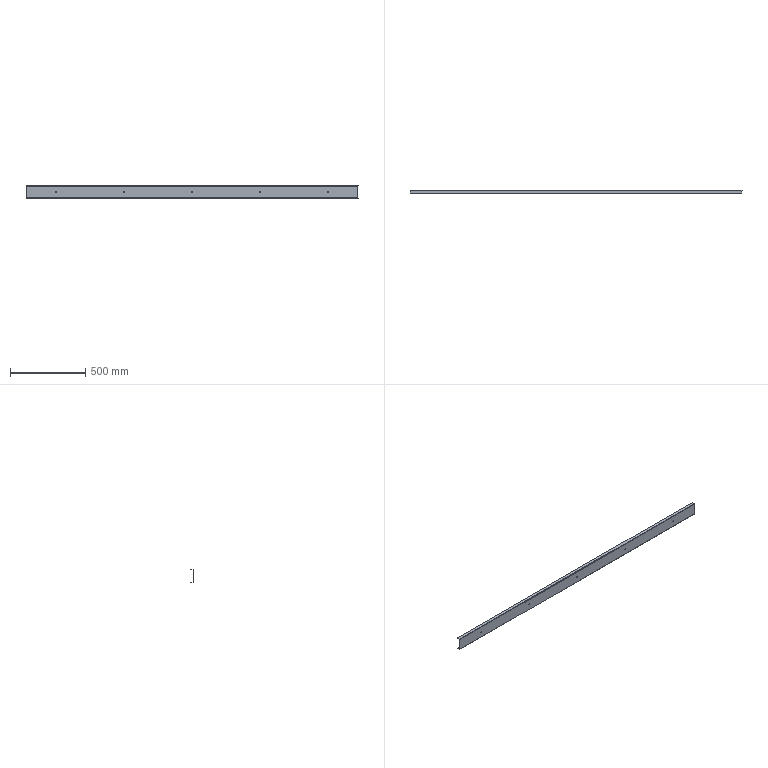Part | SolidWorks | features EdgeFlange 1, FlatPattern 1, HoleWzd 1, SMBaseFlange 1, SheetMetal 1 | 1 solid | 32 faces | box 2200 x 22 x 84 mm | volume 538758 mm3 | plane 18 | cylinder 14 | commonest cylinder face diameters 6 x10 1.473 x2 5.473 x2
STEP:
#1=CARTESIAN_POINT('',(900.,-2.,-3.));
#2=VERTEX_POINT('',#1);
#3=CARTESIAN_POINT('',(900.,-2.,3.));
#4=VERTEX_POINT('',#3);
#5=CARTESIAN_POINT('',(900.,-2.,0.));
#6=DIRECTION('',(0.,1.,0.));
#7=DIRECTION('',(0.,0.,1.));
#8=AXIS2_PLACEMENT_3D('',#5,#6,#7);
#9=CIRCLE('',#8,3.);
#10=EDGE_CURVE('',#2,#4,#9,.T.);
#11=ORIENTED_EDGE('',*,*,#10,.F.);
#12=CARTESIAN_POINT('',(900.,0.,-3.));
#13=VERTEX_POINT('',#12);
#14=CARTESIAN_POINT('',(900.,0.,-3.));
#15=DIRECTION('',(0.,1.,0.));
#16=VECTOR('',#15,1000.);
#17=LINE('',#14,#16);
#18=EDGE_CURVE('',#2,#13,#17,.T.);
#19=ORIENTED_EDGE('',*,*,#18,.T.);
#20=CARTESIAN_POINT('',(900.,0.,3.));
#21=VERTEX_POINT('',#20);
#22=CARTESIAN_POINT('',(900.,0.,0.));
#23=DIRECTION('',(0.,1.,0.));
#24=DIRECTION('',(0.,0.,1.));
#25=AXIS2_PLACEMENT_3D('',#22,#23,#24);
#26=CIRCLE('',#25,3.);
#27=EDGE_CURVE('',#13,#21,#26,.T.);
#28=ORIENTED_EDGE('',*,*,#27,.T.);
#29=CARTESIAN_POINT('',(900.,0.,3.));
#30=DIRECTION('',(0.,1.,0.));
#31=VECTOR('',#30,1000.);
#32=LINE('',#29,#31);
#33=EDGE_CURVE('',#4,#21,#32,.T.);
#34=ORIENTED_EDGE('',*,*,#33,.F.);
#35=EDGE_LOOP('',(#11,#19,#28,#34));
#36=FACE_OUTER_BOUND('',#35,.T.);
#37=CARTESIAN_POINT('',(900.,0.,0.));
#38=DIRECTION('',(0.,1.,0.));
#39=DIRECTION('',(0.,0.,1.));
#40=AXIS2_PLACEMENT_3D('',#37,#38,#39);
#41=CYLINDRICAL_SURFACE('',#40,3.);
#42=ADVANCED_FACE('',(#36),#41,.F.);
#43=CARTESIAN_POINT('',(450.,-2.,-3.));
#44=VERTEX_POINT('',#43);
#45=CARTESIAN_POINT('',(450.,-2.,3.));
#46=VERTEX_POINT('',#45);
#47=CARTESIAN_POINT('',(450.,-2.,0.));
#48=DIRECTION('',(0.,1.,0.));
#49=DIRECTION('',(0.,0.,1.));
#50=AXIS2_PLACEMENT_3D('',#47,#48,#49);
#51=CIRCLE('',#50,3.);
#52=EDGE_CURVE('',#44,#46,#51,.T.);
#53=ORIENTED_EDGE('',*,*,#52,.F.);
#54=CARTESIAN_POINT('',(450.,0.,-3.));
#55=VERTEX_POINT('',#54);
#56=CARTESIAN_POINT('',(450.,0.,-3.));
#57=DIRECTION('',(0.,1.,0.));
#58=VECTOR('',#57,1000.);
#59=LINE('',#56,#58);
#60=EDGE_CURVE('',#44,#55,#59,.T.);
#61=ORIENTED_EDGE('',*,*,#60,.T.);
#62=CARTESIAN_POINT('',(450.,0.,3.));
#63=VERTEX_POINT('',#62);
#64=CARTESIAN_POINT('',(450.,0.,0.));
#65=DIRECTION('',(0.,1.,0.));
#66=DIRECTION('',(0.,0.,1.));
#67=AXIS2_PLACEMENT_3D('',#64,#65,#66);
#68=CIRCLE('',#67,3.);
#69=EDGE_CURVE('',#55,#63,#68,.T.);
#70=ORIENTED_EDGE('',*,*,#69,.T.);
#71=CARTESIAN_POINT('',(450.,0.,3.));
#72=DIRECTION('',(0.,1.,0.));
#73=VECTOR('',#72,1000.);
#74=LINE('',#71,#73);
#75=EDGE_CURVE('',#46,#63,#74,.T.);
#76=ORIENTED_EDGE('',*,*,#75,.F.);
#77=EDGE_LOOP('',(#53,#61,#70,#76));
#78=FACE_OUTER_BOUND('',#77,.T.);
#79=CARTESIAN_POINT('',(450.,0.,0.));
#80=DIRECTION('',(0.,1.,0.));
#81=DIRECTION('',(0.,0.,1.));
#82=AXIS2_PLACEMENT_3D('',#79,#80,#81);
#83=CYLINDRICAL_SURFACE('',#82,3.);
#84=ADVANCED_FACE('',(#78),#83,.F.);
#85=CARTESIAN_POINT('',(0.,-2.,-3.));
#86=VERTEX_POINT('',#85);
#87=CARTESIAN_POINT('',(0.,-2.,3.));
#88=VERTEX_POINT('',#87);
#89=CARTESIAN_POINT('',(0.,-2.,0.));
#90=DIRECTION('',(0.,1.,0.));
#91=DIRECTION('',(0.,0.,1.));
#92=AXIS2_PLACEMENT_3D('',#89,#90,#91);
#93=CIRCLE('',#92,3.);
#94=EDGE_CURVE('',#86,#88,#93,.T.);
#95=ORIENTED_EDGE('',*,*,#94,.F.);
#96=CARTESIAN_POINT('',(0.,0.,-3.));
#97=VERTEX_POINT('',#96);
#98=CARTESIAN_POINT('',(0.,0.,-3.));
#99=DIRECTION('',(0.,1.,0.));
#100=VECTOR('',#99,1000.);
#101=LINE('',#98,#100);
#102=EDGE_CURVE('',#86,#97,#101,.T.);
#103=ORIENTED_EDGE('',*,*,#102,.T.);
#104=CARTESIAN_POINT('',(0.,0.,3.));
#105=VERTEX_POINT('',#104);
#106=CARTESIAN_POINT('',(0.,0.,0.));
#107=DIRECTION('',(0.,1.,0.));
#108=DIRECTION('',(0.,0.,1.));
#109=AXIS2_PLACEMENT_3D('',#106,#107,#108);
#110=CIRCLE('',#109,3.);
#111=EDGE_CURVE('',#97,#105,#110,.T.);
#112=ORIENTED_EDGE('',*,*,#111,.T.);
#113=CARTESIAN_POINT('',(0.,0.,3.));
#114=DIRECTION('',(0.,1.,0.));
#115=VECTOR('',#114,1000.);
#116=LINE('',#113,#115);
#117=EDGE_CURVE('',#88,#105,#116,.T.);
#118=ORIENTED_EDGE('',*,*,#117,.F.);
#119=EDGE_LOOP('',(#95,#103,#112,#118));
#120=FACE_OUTER_BOUND('',#119,.T.);
#121=CARTESIAN_POINT('',(0.,0.,0.));
#122=DIRECTION('',(0.,1.,0.));
#123=DIRECTION('',(0.,0.,1.));
#124=AXIS2_PLACEMENT_3D('',#121,#122,#123);
#125=CYLINDRICAL_SURFACE('',#124,3.);
#126=ADVANCED_FACE('',(#120),#125,.F.);
#127=CARTESIAN_POINT('',(-450.,-2.,-3.));
#128=VERTEX_POINT('',#127);
#129=CARTESIAN_POINT('',(-450.,-2.,3.));
#130=VERTEX_POINT('',#129);
#131=CARTESIAN_POINT('',(-450.,-2.,0.));
#132=DIRECTION('',(0.,1.,0.));
#133=DIRECTION('',(0.,0.,1.));
#134=AXIS2_PLACEMENT_3D('',#131,#132,#133);
#135=CIRCLE('',#134,3.);
#136=EDGE_CURVE('',#128,#130,#135,.T.);
#137=ORIENTED_EDGE('',*,*,#136,.F.);
#138=CARTESIAN_POINT('',(-450.,0.,-3.));
#139=VERTEX_POINT('',#138);
#140=CARTESIAN_POINT('',(-450.,0.,-3.));
#141=DIRECTION('',(0.,1.,0.));
#142=VECTOR('',#141,1000.);
#143=LINE('',#140,#142);
#144=EDGE_CURVE('',#128,#139,#143,.T.);
#145=ORIENTED_EDGE('',*,*,#144,.T.);
#146=CARTESIAN_POINT('',(-450.,0.,3.));
#147=VERTEX_POINT('',#146);
#148=CARTESIAN_POINT('',(-450.,0.,0.));
#149=DIRECTION('',(0.,1.,0.));
#150=DIRECTION('',(0.,0.,1.));
#151=AXIS2_PLACEMENT_3D('',#148,#149,#150);
#152=CIRCLE('',#151,3.);
#153=EDGE_CURVE('',#139,#147,#152,.T.);
#154=ORIENTED_EDGE('',*,*,#153,.T.);
#155=CARTESIAN_POINT('',(-450.,0.,3.));
#156=DIRECTION('',(0.,1.,0.));
#157=VECTOR('',#156,1000.);
#158=LINE('',#155,#157);
#159=EDGE_CURVE('',#130,#147,#158,.T.);
#160=ORIENTED_EDGE('',*,*,#159,.F.);
#161=EDGE_LOOP('',(#137,#145,#154,#160));
#162=FACE_OUTER_BOUND('',#161,.T.);
#163=CARTESIAN_POINT('',(-450.,0.,0.));
#164=DIRECTION('',(0.,1.,0.));
#165=DIRECTION('',(0.,0.,1.));
#166=AXIS2_PLACEMENT_3D('',#163,#164,#165);
#167=CYLINDRICAL_SURFACE('',#166,3.);
#168=ADVANCED_FACE('',(#162),#167,.F.);
#169=CARTESIAN_POINT('',(-900.,-2.,-3.));
#170=VERTEX_POINT('',#169);
#171=CARTESIAN_POINT('',(-900.,-2.,3.));
#172=VERTEX_POINT('',#171);
#173=CARTESIAN_POINT('',(-900.,-2.,0.));
#174=DIRECTION('',(0.,1.,0.));
#175=DIRECTION('',(0.,0.,1.));
#176=AXIS2_PLACEMENT_3D('',#173,#174,#175);
#177=CIRCLE('',#176,3.);
#178=EDGE_CURVE('',#170,#172,#177,.T.);
#179=ORIENTED_EDGE('',*,*,#178,.F.);
#180=CARTESIAN_POINT('',(-900.,0.,-3.));
#181=VERTEX_POINT('',#180);
#182=CARTESIAN_POINT('',(-900.,0.,-3.));
#183=DIRECTION('',(0.,1.,0.));
#184=VECTOR('',#183,1000.);
#185=LINE('',#182,#184);
#186=EDGE_CURVE('',#170,#181,#185,.T.);
#187=ORIENTED_EDGE('',*,*,#186,.T.);
#188=CARTESIAN_POINT('',(-900.,0.,3.));
#189=VERTEX_POINT('',#188);
#190=CARTESIAN_POINT('',(-900.,0.,0.));
#191=DIRECTION('',(0.,1.,0.));
#192=DIRECTION('',(0.,0.,1.));
#193=AXIS2_PLACEMENT_3D('',#190,#191,#192);
#194=CIRCLE('',#193,3.);
#195=EDGE_CURVE('',#181,#189,#194,.T.);
#196=ORIENTED_EDGE('',*,*,#195,.T.);
#197=CARTESIAN_POINT('',(-900.,0.,3.));
#198=DIRECTION('',(0.,1.,0.));
#199=VECTOR('',#198,1000.);
#200=LINE('',#197,#199);
#201=EDGE_CURVE('',#172,#189,#200,.T.);
#202=ORIENTED_EDGE('',*,*,#201,.F.);
#203=EDGE_LOOP('',(#179,#187,#196,#202));
#204=FACE_OUTER_BOUND('',#203,.T.);
#205=CARTESIAN_POINT('',(-900.,0.,0.));
#206=DIRECTION('',(0.,1.,0.));
#207=DIRECTION('',(0.,0.,1.));
#208=AXIS2_PLACEMENT_3D('',#205,#206,#207);
#209=CYLINDRICAL_SURFACE('',#208,3.);
#210=ADVANCED_FACE('',(#204),#209,.F.);
#211=CARTESIAN_POINT('',(900.,-2.,0.));
#212=DIRECTION('',(0.,1.,0.));
#213=DIRECTION('',(0.,0.,1.));
#214=AXIS2_PLACEMENT_3D('',#211,#212,#213);
#215=CIRCLE('',#214,3.);
#216=EDGE_CURVE('',#4,#2,#215,.T.);
#217=ORIENTED_EDGE('',*,*,#216,.T.);
#218=ORIENTED_EDGE('',*,*,#10,.T.);
#219=EDGE_LOOP('',(#217,#218));
#220=FACE_BOUND('',#219,.T.);
#221=CARTESIAN_POINT('',(450.,-2.,0.));
#222=DIRECTION('',(0.,1.,0.));
#223=DIRECTION('',(0.,0.,1.));
#224=AXIS2_PLACEMENT_3D('',#221,#222,#223);
#225=CIRCLE('',#224,3.);
#226=EDGE_CURVE('',#46,#44,#225,.T.);
#227=ORIENTED_EDGE('',*,*,#226,.T.);
#228=ORIENTED_EDGE('',*,*,#52,.T.);
#229=EDGE_LOOP('',(#227,#228));
#230=FACE_BOUND('',#229,.T.);
#231=CARTESIAN_POINT('',(0.,-2.,0.));
#232=DIRECTION('',(0.,1.,0.));
#233=DIRECTION('',(0.,0.,1.));
#234=AXIS2_PLACEMENT_3D('',#231,#232,#233);
#235=CIRCLE('',#234,3.);
#236=EDGE_CURVE('',#88,#86,#235,.T.);
#237=ORIENTED_EDGE('',*,*,#236,.T.);
#238=ORIENTED_EDGE('',*,*,#94,.T.);
#239=EDGE_LOOP('',(#237,#238));
#240=FACE_BOUND('',#239,.T.);
#241=CARTESIAN_POINT('',(-450.,-2.,0.));
#242=DIRECTION('',(0.,1.,0.));
#243=DIRECTION('',(0.,0.,1.));
#244=AXIS2_PLACEMENT_3D('',#241,#242,#243);
#245=CIRCLE('',#244,3.);
#246=EDGE_CURVE('',#130,#128,#245,.T.);
#247=ORIENTED_EDGE('',*,*,#246,.T.);
#248=ORIENTED_EDGE('',*,*,#136,.T.);
#249=EDGE_LOOP('',(#247,#248));
#250=FACE_BOUND('',#249,.T.);
#251=CARTESIAN_POINT('',(-900.,-2.,0.));
#252=DIRECTION('',(0.,1.,0.));
#253=DIRECTION('',(0.,0.,1.));
#254=AXIS2_PLACEMENT_3D('',#251,#252,#253);
#255=CIRCLE('',#254,3.);
#256=EDGE_CURVE('',#172,#170,#255,.T.);
#257=ORIENTED_EDGE('',*,*,#256,.T.);
#258=ORIENTED_EDGE('',*,*,#178,.T.);
#259=EDGE_LOOP('',(#257,#258));
#260=FACE_BOUND('',#259,.T.);
#261=CARTESIAN_POINT('',(-1100.,-2.,-39.263));
#262=VERTEX_POINT('',#261);
#263=CARTESIAN_POINT('',(1100.,-2.,-39.263));
#264=VERTEX_POINT('',#263);
#265=CARTESIAN_POINT('',(-1100.,-2.,-39.263));
#266=DIRECTION('',(1.,0.,0.));
#267=VECTOR('',#266,1000.);
#268=LINE('',#265,#267);
#269=EDGE_CURVE('',#262,#264,#268,.T.);
#270=ORIENTED_EDGE('',*,*,#269,.T.);
#271=CARTESIAN_POINT('',(1100.,-2.,39.263));
#272=VERTEX_POINT('',#271);
#273=CARTESIAN_POINT('',(1100.,-2.,-42.));
#274=DIRECTION('',(0.,0.,-1.));
#275=VECTOR('',#274,1000.);
#276=LINE('',#273,#275);
#277=EDGE_CURVE('',#272,#264,#276,.T.);
#278=ORIENTED_EDGE('',*,*,#277,.F.);
#279=CARTESIAN_POINT('',(-1100.,-2.,39.263));
#280=VERTEX_POINT('',#279);
#281=CARTESIAN_POINT('',(1100.,-2.,39.263));
#282=DIRECTION('',(-1.,0.,0.));
#283=VECTOR('',#282,1000.);
#284=LINE('',#281,#283);
#285=EDGE_CURVE('',#272,#280,#284,.T.);
#286=ORIENTED_EDGE('',*,*,#285,.T.);
#287=CARTESIAN_POINT('',(-1100.,-2.,-42.));
#288=DIRECTION('',(0.,0.,1.));
#289=VECTOR('',#288,1000.);
#290=LINE('',#287,#289);
#291=EDGE_CURVE('',#262,#280,#290,.T.);
#292=ORIENTED_EDGE('',*,*,#291,.F.);
#293=EDGE_LOOP('',(#270,#278,#286,#292));
#294=FACE_OUTER_BOUND('',#293,.T.);
#295=CARTESIAN_POINT('',(0.,-2.,0.));
#296=DIRECTION('',(0.,1.,0.));
#297=DIRECTION('',(0.,0.,1.));
#298=AXIS2_PLACEMENT_3D('',#295,#296,#297);
#299=PLANE('',#298);
#300=ADVANCED_FACE('',(#220,#230,#240,#250,#260,#294),#299,.F.);
#301=CARTESIAN_POINT('',(900.,0.,0.));
#302=DIRECTION('',(0.,1.,0.));
#303=DIRECTION('',(0.,0.,1.));
#304=AXIS2_PLACEMENT_3D('',#301,#302,#303);
#305=CIRCLE('',#304,3.);
#306=EDGE_CURVE('',#21,#13,#305,.T.);
#307=ORIENTED_EDGE('',*,*,#306,.F.);
#308=ORIENTED_EDGE('',*,*,#27,.F.);
#309=EDGE_LOOP('',(#307,#308));
#310=FACE_BOUND('',#309,.T.);
#311=CARTESIAN_POINT('',(450.,0.,0.));
#312=DIRECTION('',(0.,1.,0.));
#313=DIRECTION('',(0.,0.,1.));
#314=AXIS2_PLACEMENT_3D('',#311,#312,#313);
#315=CIRCLE('',#314,3.);
#316=EDGE_CURVE('',#63,#55,#315,.T.);
#317=ORIENTED_EDGE('',*,*,#316,.F.);
#318=ORIENTED_EDGE('',*,*,#69,.F.);
#319=EDGE_LOOP('',(#317,#318));
#320=FACE_BOUND('',#319,.T.);
#321=CARTESIAN_POINT('',(0.,0.,0.));
#322=DIRECTION('',(0.,1.,0.));
#323=DIRECTION('',(0.,0.,1.));
#324=AXIS2_PLACEMENT_3D('',#321,#322,#323);
#325=CIRCLE('',#324,3.);
#326=EDGE_CURVE('',#105,#97,#325,.T.);
#327=ORIENTED_EDGE('',*,*,#326,.F.);
#328=ORIENTED_EDGE('',*,*,#111,.F.);
#329=EDGE_LOOP('',(#327,#328));
#330=FACE_BOUND('',#329,.T.);
#331=CARTESIAN_POINT('',(-450.,0.,0.));
#332=DIRECTION('',(0.,1.,0.));
#333=DIRECTION('',(0.,0.,1.));
#334=AXIS2_PLACEMENT_3D('',#331,#332,#333);
#335=CIRCLE('',#334,3.);
#336=EDGE_CURVE('',#147,#139,#335,.T.);
#337=ORIENTED_EDGE('',*,*,#336,.F.);
#338=ORIENTED_EDGE('',*,*,#153,.F.);
#339=EDGE_LOOP('',(#337,#338));
#340=FACE_BOUND('',#339,.T.);
#341=CARTESIAN_POINT('',(-900.,0.,0.));
#342=DIRECTION('',(0.,1.,0.));
#343=DIRECTION('',(0.,0.,1.));
#344=AXIS2_PLACEMENT_3D('',#341,#342,#343);
#345=CIRCLE('',#344,3.);
#346=EDGE_CURVE('',#189,#181,#345,.T.);
#347=ORIENTED_EDGE('',*,*,#346,.F.);
#348=ORIENTED_EDGE('',*,*,#195,.F.);
#349=EDGE_LOOP('',(#347,#348));
#350=FACE_BOUND('',#349,.T.);
#351=CARTESIAN_POINT('',(1100.,0.,39.263));
#352=VERTEX_POINT('',#351);
#353=CARTESIAN_POINT('',(1100.,0.,-39.263));
#354=VERTEX_POINT('',#353);
#355=CARTESIAN_POINT('',(1100.,0.,-42.));
#356=DIRECTION('',(0.,0.,-1.));
#357=VECTOR('',#356,1000.);
#358=LINE('',#355,#357);
#359=EDGE_CURVE('',#352,#354,#358,.T.);
#360=ORIENTED_EDGE('',*,*,#359,.T.);
#361=CARTESIAN_POINT('',(-1100.,0.,-39.263));
#362=VERTEX_POINT('',#361);
#363=CARTESIAN_POINT('',(-1100.,0.,-39.263));
#364=DIRECTION('',(1.,0.,0.));
#365=VECTOR('',#364,1000.);
#366=LINE('',#363,#365);
#367=EDGE_CURVE('',#362,#354,#366,.T.);
#368=ORIENTED_EDGE('',*,*,#367,.F.);
#369=CARTESIAN_POINT('',(-1100.,0.,39.263));
#370=VERTEX_POINT('',#369);
#371=CARTESIAN_POINT('',(-1100.,0.,-42.));
#372=DIRECTION('',(0.,0.,1.));
#373=VECTOR('',#372,1000.);
#374=LINE('',#371,#373);
#375=EDGE_CURVE('',#362,#370,#374,.T.);
#376=ORIENTED_EDGE('',*,*,#375,.T.);
#377=CARTESIAN_POINT('',(1100.,0.,39.263));
#378=DIRECTION('',(-1.,0.,0.));
#379=VECTOR('',#378,1000.);
#380=LINE('',#377,#379);
#381=EDGE_CURVE('',#352,#370,#380,.T.);
#382=ORIENTED_EDGE('',*,*,#381,.F.);
#383=EDGE_LOOP('',(#360,#368,#376,#382));
#384=FACE_OUTER_BOUND('',#383,.T.);
#385=CARTESIAN_POINT('',(0.,0.,0.));
#386=DIRECTION('',(0.,1.,0.));
#387=DIRECTION('',(0.,0.,1.));
#388=AXIS2_PLACEMENT_3D('',#385,#386,#387);
#389=PLANE('',#388);
#390=ADVANCED_FACE('',(#310,#320,#330,#340,#350,#384),#389,.T.);
#391=ORIENTED_EDGE('',*,*,#375,.F.);
#392=CARTESIAN_POINT('',(-1100.,0.,-39.263));
#393=DIRECTION('',(0.,-1.,0.));
#394=VECTOR('',#393,1000.);
#395=LINE('',#392,#394);
#396=EDGE_CURVE('',#362,#262,#395,.T.);
#397=ORIENTED_EDGE('',*,*,#396,.T.);
#398=ORIENTED_EDGE('',*,*,#291,.T.);
#399=CARTESIAN_POINT('',(-1100.,0.,39.263));
#400=DIRECTION('',(0.,-1.,0.));
#401=VECTOR('',#400,1000.);
#402=LINE('',#399,#401);
#403=EDGE_CURVE('',#370,#280,#402,.T.);
#404=ORIENTED_EDGE('',*,*,#403,.F.);
#405=EDGE_LOOP('',(#391,#397,#398,#404));
#406=FACE_OUTER_BOUND('',#405,.T.);
#407=CARTESIAN_POINT('',(-1100.,-2.,-42.));
#408=DIRECTION('',(-1.,0.,0.));
#409=DIRECTION('',(0.,0.,1.));
#410=AXIS2_PLACEMENT_3D('',#407,#408,#409);
#411=PLANE('',#410);
#412=ADVANCED_FACE('',(#406),#411,.T.);
#413=CARTESIAN_POINT('',(1100.,0.,-39.263));
#414=DIRECTION('',(0.,-1.,0.));
#415=VECTOR('',#414,1000.);
#416=LINE('',#413,#415);
#417=EDGE_CURVE('',#354,#264,#416,.T.);
#418=ORIENTED_EDGE('',*,*,#417,.F.);
#419=ORIENTED_EDGE('',*,*,#359,.F.);
#420=CARTESIAN_POINT('',(1100.,0.,39.263));
#421=DIRECTION('',(0.,-1.,0.));
#422=VECTOR('',#421,1000.);
#423=LINE('',#420,#422);
#424=EDGE_CURVE('',#352,#272,#423,.T.);
#425=ORIENTED_EDGE('',*,*,#424,.T.);
#426=ORIENTED_EDGE('',*,*,#277,.T.);
#427=EDGE_LOOP('',(#418,#419,#425,#426));
#428=FACE_OUTER_BOUND('',#427,.T.);
#429=CARTESIAN_POINT('',(1100.,-2.,-42.));
#430=DIRECTION('',(1.,0.,0.));
#431=DIRECTION('',(0.,0.,-1.));
#432=AXIS2_PLACEMENT_3D('',#429,#430,#431);
#433=PLANE('',#432);
#434=ADVANCED_FACE('',(#428),#433,.T.);
#435=CARTESIAN_POINT('',(-1100.,0.7366,40.));
#436=VERTEX_POINT('',#435);
#437=CARTESIAN_POINT('',(-1100.,0.7366,42.));
#438=VERTEX_POINT('',#437);
#439=CARTESIAN_POINT('',(-1100.,0.7366,42.));
#440=DIRECTION('',(0.,0.,1.));
#441=VECTOR('',#440,1000.);
#442=LINE('',#439,#441);
#443=EDGE_CURVE('',#436,#438,#442,.T.);
#444=ORIENTED_EDGE('',*,*,#443,.F.);
#445=CARTESIAN_POINT('',(-1100.,0.7366,39.263));
#446=DIRECTION('',(-1.,0.,0.));
#447=DIRECTION('',(0.,0.,-1.));
#448=AXIS2_PLACEMENT_3D('',#445,#446,#447);
#449=CIRCLE('',#448,0.7366);
#450=EDGE_CURVE('',#370,#436,#449,.T.);
#451=ORIENTED_EDGE('',*,*,#450,.F.);
#452=ORIENTED_EDGE('',*,*,#403,.T.);
#453=CARTESIAN_POINT('',(-1100.,0.7366,39.263));
#454=DIRECTION('',(-1.,0.,0.));
#455=DIRECTION('',(0.,0.,-1.));
#456=AXIS2_PLACEMENT_3D('',#453,#454,#455);
#457=CIRCLE('',#456,2.737);
#458=EDGE_CURVE('',#280,#438,#457,.T.);
#459=ORIENTED_EDGE('',*,*,#458,.T.);
#460=EDGE_LOOP('',(#444,#451,#452,#459));
#461=FACE_OUTER_BOUND('',#460,.T.);
#462=CARTESIAN_POINT('',(-1100.,0.7366,39.263));
#463=DIRECTION('',(-1.,0.,0.));
#464=DIRECTION('',(0.,0.,1.));
#465=AXIS2_PLACEMENT_3D('',#462,#463,#464);
#466=PLANE('',#465);
#467=ADVANCED_FACE('',(#461),#466,.T.);
#468=CARTESIAN_POINT('',(1100.,0.7366,40.));
#469=VERTEX_POINT('',#468);
#470=CARTESIAN_POINT('',(1100.,0.7366,39.263));
#471=DIRECTION('',(1.,0.,0.));
#472=DIRECTION('',(0.,0.,-1.));
#473=AXIS2_PLACEMENT_3D('',#470,#471,#472);
#474=CIRCLE('',#473,0.7366);
#475=EDGE_CURVE('',#469,#352,#474,.T.);
#476=ORIENTED_EDGE('',*,*,#475,.F.);
#477=CARTESIAN_POINT('',(1100.,0.7366,42.));
#478=VERTEX_POINT('',#477);
#479=CARTESIAN_POINT('',(1100.,0.7366,40.));
#480=DIRECTION('',(0.,0.,1.));
#481=VECTOR('',#480,1000.);
#482=LINE('',#479,#481);
#483=EDGE_CURVE('',#469,#478,#482,.T.);
#484=ORIENTED_EDGE('',*,*,#483,.T.);
#485=CARTESIAN_POINT('',(1100.,0.7366,39.263));
#486=DIRECTION('',(1.,0.,0.));
#487=DIRECTION('',(0.,0.,-1.));
#488=AXIS2_PLACEMENT_3D('',#485,#486,#487);
#489=CIRCLE('',#488,2.737);
#490=EDGE_CURVE('',#478,#272,#489,.T.);
#491=ORIENTED_EDGE('',*,*,#490,.T.);
#492=ORIENTED_EDGE('',*,*,#424,.F.);
#493=EDGE_LOOP('',(#476,#484,#491,#492));
#494=FACE_OUTER_BOUND('',#493,.T.);
#495=CARTESIAN_POINT('',(1100.,0.7366,39.263));
#496=DIRECTION('',(-1.,0.,0.));
#497=DIRECTION('',(0.,0.,1.));
#498=AXIS2_PLACEMENT_3D('',#495,#496,#497);
#499=PLANE('',#498);
#500=ADVANCED_FACE('',(#494),#499,.F.);
#501=ORIENTED_EDGE('',*,*,#285,.F.);
#502=ORIENTED_EDGE('',*,*,#490,.F.);
#503=CARTESIAN_POINT('',(-1100.,0.7366,42.));
#504=DIRECTION('',(-1.,0.,0.));
#505=VECTOR('',#504,1000.);
#506=LINE('',#503,#505);
#507=EDGE_CURVE('',#478,#438,#506,.T.);
#508=ORIENTED_EDGE('',*,*,#507,.T.);
#509=ORIENTED_EDGE('',*,*,#458,.F.);
#510=EDGE_LOOP('',(#501,#502,#508,#509));
#511=FACE_OUTER_BOUND('',#510,.T.);
#512=CARTESIAN_POINT('',(1100.,0.7366,39.263));
#513=DIRECTION('',(1.,0.,0.));
#514=DIRECTION('',(0.,0.,1.));
#515=AXIS2_PLACEMENT_3D('',#512,#513,#514);
#516=CYLINDRICAL_SURFACE('',#515,2.737);
#517=ADVANCED_FACE('',(#511),#516,.T.);
#518=ORIENTED_EDGE('',*,*,#381,.T.);
#519=ORIENTED_EDGE('',*,*,#450,.T.);
#520=CARTESIAN_POINT('',(-1100.,0.7366,40.));
#521=DIRECTION('',(1.,0.,0.));
#522=VECTOR('',#521,1000.);
#523=LINE('',#520,#522);
#524=EDGE_CURVE('',#436,#469,#523,.T.);
#525=ORIENTED_EDGE('',*,*,#524,.T.);
#526=ORIENTED_EDGE('',*,*,#475,.T.);
#527=EDGE_LOOP('',(#518,#519,#525,#526));
#528=FACE_OUTER_BOUND('',#527,.T.);
#529=CARTESIAN_POINT('',(1100.,0.7366,39.263));
#530=DIRECTION('',(1.,0.,0.));
#531=DIRECTION('',(0.,0.,1.));
#532=AXIS2_PLACEMENT_3D('',#529,#530,#531);
#533=CYLINDRICAL_SURFACE('',#532,0.7366);
#534=ADVANCED_FACE('',(#528),#533,.F.);
#535=ORIENTED_EDGE('',*,*,#443,.T.);
#536=CARTESIAN_POINT('',(-1100.,20.,42.));
#537=VERTEX_POINT('',#536);
#538=CARTESIAN_POINT('',(-1100.,0.,42.));
#539=DIRECTION('',(0.,-1.,0.));
#540=VECTOR('',#539,1000.);
#541=LINE('',#538,#540);
#542=EDGE_CURVE('',#537,#438,#541,.T.);
#543=ORIENTED_EDGE('',*,*,#542,.F.);
#544=CARTESIAN_POINT('',(-1100.,20.,40.));
#545=VERTEX_POINT('',#544);
#546=CARTESIAN_POINT('',(-1100.,20.,42.));
#547=DIRECTION('',(0.,0.,-1.));
#548=VECTOR('',#547,1000.);
#549=LINE('',#546,#548);
#550=EDGE_CURVE('',#537,#545,#549,.T.);
#551=ORIENTED_EDGE('',*,*,#550,.T.);
#552=CARTESIAN_POINT('',(-1100.,0.,40.));
#553=DIRECTION('',(0.,-1.,0.));
#554=VECTOR('',#553,1000.);
#555=LINE('',#552,#554);
#556=EDGE_CURVE('',#545,#436,#555,.T.);
#557=ORIENTED_EDGE('',*,*,#556,.T.);
#558=EDGE_LOOP('',(#535,#543,#551,#557));
#559=FACE_OUTER_BOUND('',#558,.T.);
#560=CARTESIAN_POINT('',(-1100.,0.,42.));
#561=DIRECTION('',(1.,0.,0.));
#562=DIRECTION('',(0.,1.,0.));
#563=AXIS2_PLACEMENT_3D('',#560,#561,#562);
#564=PLANE('',#563);
#565=ADVANCED_FACE('',(#559),#564,.F.);
#566=ORIENTED_EDGE('',*,*,#483,.F.);
#567=CARTESIAN_POINT('',(1100.,20.,40.));
#568=VERTEX_POINT('',#567);
#569=CARTESIAN_POINT('',(1100.,20.,40.));
#570=DIRECTION('',(0.,1.,0.));
#571=VECTOR('',#570,1000.);
#572=LINE('',#569,#571);
#573=EDGE_CURVE('',#469,#568,#572,.T.);
#574=ORIENTED_EDGE('',*,*,#573,.T.);
#575=CARTESIAN_POINT('',(1100.,20.,42.));
#576=VERTEX_POINT('',#575);
#577=CARTESIAN_POINT('',(1100.,20.,42.));
#578=DIRECTION('',(0.,0.,-1.));
#579=VECTOR('',#578,1000.);
#580=LINE('',#577,#579);
#581=EDGE_CURVE('',#576,#568,#580,.T.);
#582=ORIENTED_EDGE('',*,*,#581,.F.);
#583=CARTESIAN_POINT('',(1100.,0.,42.));
#584=DIRECTION('',(0.,1.,0.));
#585=VECTOR('',#584,1000.);
#586=LINE('',#583,#585);
#587=EDGE_CURVE('',#478,#576,#586,.T.);
#588=ORIENTED_EDGE('',*,*,#587,.F.);
#589=EDGE_LOOP('',(#566,#574,#582,#588));
#590=FACE_OUTER_BOUND('',#589,.T.);
#591=CARTESIAN_POINT('',(1100.,20.,42.));
#592=DIRECTION('',(-1.,0.,0.));
#593=DIRECTION('',(0.,-1.,0.));
#594=AXIS2_PLACEMENT_3D('',#591,#592,#593);
#595=PLANE('',#594);
#596=ADVANCED_FACE('',(#590),#595,.F.);
#597=ORIENTED_EDGE('',*,*,#507,.F.);
#598=ORIENTED_EDGE('',*,*,#587,.T.);
#599=CARTESIAN_POINT('',(0.,20.,42.));
#600=DIRECTION('',(-1.,0.,0.));
#601=VECTOR('',#600,1000.);
#602=LINE('',#599,#601);
#603=EDGE_CURVE('',#576,#537,#602,.T.);
#604=ORIENTED_EDGE('',*,*,#603,.T.);
#605=ORIENTED_EDGE('',*,*,#542,.T.);
#606=EDGE_LOOP('',(#597,#598,#604,#605));
#607=FACE_OUTER_BOUND('',#606,.T.);
#608=CARTESIAN_POINT('',(0.,0.,42.));
#609=DIRECTION('',(0.,0.,-1.));
#610=DIRECTION('',(-1.,0.,0.));
#611=AXIS2_PLACEMENT_3D('',#608,#609,#610);
#612=PLANE('',#611);
#613=ADVANCED_FACE('',(#607),#612,.F.);
#614=ORIENTED_EDGE('',*,*,#573,.F.);
#615=ORIENTED_EDGE('',*,*,#524,.F.);
#616=ORIENTED_EDGE('',*,*,#556,.F.);
#617=CARTESIAN_POINT('',(-1100.,20.,40.));
#618=DIRECTION('',(-1.,0.,0.));
#619=VECTOR('',#618,1000.);
#620=LINE('',#617,#619);
#621=EDGE_CURVE('',#568,#545,#620,.T.);
#622=ORIENTED_EDGE('',*,*,#621,.F.);
#623=EDGE_LOOP('',(#614,#615,#616,#622));
#624=FACE_OUTER_BOUND('',#623,.T.);
#625=CARTESIAN_POINT('',(0.,0.,40.));
#626=DIRECTION('',(0.,0.,-1.));
#627=DIRECTION('',(-1.,0.,0.));
#628=AXIS2_PLACEMENT_3D('',#625,#626,#627);
#629=PLANE('',#628);
#630=ADVANCED_FACE('',(#624),#629,.T.);
#631=ORIENTED_EDGE('',*,*,#621,.T.);
#632=ORIENTED_EDGE('',*,*,#550,.F.);
#633=ORIENTED_EDGE('',*,*,#603,.F.);
#634=ORIENTED_EDGE('',*,*,#581,.T.);
#635=EDGE_LOOP('',(#631,#632,#633,#634));
#636=FACE_OUTER_BOUND('',#635,.T.);
#637=CARTESIAN_POINT('',(-1100.,20.,42.));
#638=DIRECTION('',(0.,-1.,0.));
#639=DIRECTION('',(0.,0.,-1.));
#640=AXIS2_PLACEMENT_3D('',#637,#638,#639);
#641=PLANE('',#640);
#642=ADVANCED_FACE('',(#636),#641,.F.);
#643=CARTESIAN_POINT('',(1100.,0.7366,-40.));
#644=VERTEX_POINT('',#643);
#645=CARTESIAN_POINT('',(1100.,0.7366,-42.));
#646=VERTEX_POINT('',#645);
#647=CARTESIAN_POINT('',(1100.,0.7366,-42.));
#648=DIRECTION('',(0.,0.,-1.));
#649=VECTOR('',#648,1000.);
#650=LINE('',#647,#649);
#651=EDGE_CURVE('',#644,#646,#650,.T.);
#652=ORIENTED_EDGE('',*,*,#651,.F.);
#653=CARTESIAN_POINT('',(1100.,0.7366,-39.263));
#654=DIRECTION('',(1.,0.,0.));
#655=DIRECTION('',(0.,-1.,0.));
#656=AXIS2_PLACEMENT_3D('',#653,#654,#655);
#657=CIRCLE('',#656,0.7366);
#658=EDGE_CURVE('',#354,#644,#657,.T.);
#659=ORIENTED_EDGE('',*,*,#658,.F.);
#660=ORIENTED_EDGE('',*,*,#417,.T.);
#661=CARTESIAN_POINT('',(1100.,0.7366,-39.263));
#662=DIRECTION('',(1.,0.,0.));
#663=DIRECTION('',(0.,-1.,0.));
#664=AXIS2_PLACEMENT_3D('',#661,#662,#663);
#665=CIRCLE('',#664,2.737);
#666=EDGE_CURVE('',#264,#646,#665,.T.);
#667=ORIENTED_EDGE('',*,*,#666,.T.);
#668=EDGE_LOOP('',(#652,#659,#660,#667));
#669=FACE_OUTER_BOUND('',#668,.T.);
#670=CARTESIAN_POINT('',(1100.,0.7366,-39.263));
#671=DIRECTION('',(1.,0.,0.));
#672=DIRECTION('',(0.,1.,0.));
#673=AXIS2_PLACEMENT_3D('',#670,#671,#672);
#674=PLANE('',#673);
#675=ADVANCED_FACE('',(#669),#674,.T.);
#676=CARTESIAN_POINT('',(-1100.,0.7366,-40.));
#677=VERTEX_POINT('',#676);
#678=CARTESIAN_POINT('',(-1100.,0.7366,-39.263));
#679=DIRECTION('',(-1.,0.,0.));
#680=DIRECTION('',(0.,-1.,0.));
#681=AXIS2_PLACEMENT_3D('',#678,#679,#680);
#682=CIRCLE('',#681,0.7366);
#683=EDGE_CURVE('',#677,#362,#682,.T.);
#684=ORIENTED_EDGE('',*,*,#683,.F.);
#685=CARTESIAN_POINT('',(-1100.,0.7366,-42.));
#686=VERTEX_POINT('',#685);
#687=CARTESIAN_POINT('',(-1100.,0.7366,-40.));
#688=DIRECTION('',(0.,0.,-1.));
#689=VECTOR('',#688,1000.);
#690=LINE('',#687,#689);
#691=EDGE_CURVE('',#677,#686,#690,.T.);
#692=ORIENTED_EDGE('',*,*,#691,.T.);
#693=CARTESIAN_POINT('',(-1100.,0.7366,-39.263));
#694=DIRECTION('',(-1.,0.,0.));
#695=DIRECTION('',(0.,-1.,0.));
#696=AXIS2_PLACEMENT_3D('',#693,#694,#695);
#697=CIRCLE('',#696,2.737);
#698=EDGE_CURVE('',#686,#262,#697,.T.);
#699=ORIENTED_EDGE('',*,*,#698,.T.);
#700=ORIENTED_EDGE('',*,*,#396,.F.);
#701=EDGE_LOOP('',(#684,#692,#699,#700));
#702=FACE_OUTER_BOUND('',#701,.T.);
#703=CARTESIAN_POINT('',(-1100.,0.7366,-39.263));
#704=DIRECTION('',(1.,0.,0.));
#705=DIRECTION('',(0.,1.,0.));
#706=AXIS2_PLACEMENT_3D('',#703,#704,#705);
#707=PLANE('',#706);
#708=ADVANCED_FACE('',(#702),#707,.F.);
#709=ORIENTED_EDGE('',*,*,#269,.F.);
#710=ORIENTED_EDGE('',*,*,#698,.F.);
#711=CARTESIAN_POINT('',(1100.,0.7366,-42.));
#712=DIRECTION('',(1.,0.,0.));
#713=VECTOR('',#712,1000.);
#714=LINE('',#711,#713);
#715=EDGE_CURVE('',#686,#646,#714,.T.);
#716=ORIENTED_EDGE('',*,*,#715,.T.);
#717=ORIENTED_EDGE('',*,*,#666,.F.);
#718=EDGE_LOOP('',(#709,#710,#716,#717));
#719=FACE_OUTER_BOUND('',#718,.T.);
#720=CARTESIAN_POINT('',(-1100.,0.7366,-39.263));
#721=DIRECTION('',(-1.,0.,0.));
#722=DIRECTION('',(0.,0.,-1.));
#723=AXIS2_PLACEMENT_3D('',#720,#721,#722);
#724=CYLINDRICAL_SURFACE('',#723,2.737);
#725=ADVANCED_FACE('',(#719),#724,.T.);
#726=ORIENTED_EDGE('',*,*,#367,.T.);
#727=ORIENTED_EDGE('',*,*,#658,.T.);
#728=CARTESIAN_POINT('',(1100.,0.7366,-40.));
#729=DIRECTION('',(-1.,0.,0.));
#730=VECTOR('',#729,1000.);
#731=LINE('',#728,#730);
#732=EDGE_CURVE('',#644,#677,#731,.T.);
#733=ORIENTED_EDGE('',*,*,#732,.T.);
#734=ORIENTED_EDGE('',*,*,#683,.T.);
#735=EDGE_LOOP('',(#726,#727,#733,#734));
#736=FACE_OUTER_BOUND('',#735,.T.);
#737=CARTESIAN_POINT('',(-1100.,0.7366,-39.263));
#738=DIRECTION('',(-1.,0.,0.));
#739=DIRECTION('',(0.,0.,-1.));
#740=AXIS2_PLACEMENT_3D('',#737,#738,#739);
#741=CYLINDRICAL_SURFACE('',#740,0.7366);
#742=ADVANCED_FACE('',(#736),#741,.F.);
#743=ORIENTED_EDGE('',*,*,#651,.T.);
#744=CARTESIAN_POINT('',(1100.,20.,-42.));
#745=VERTEX_POINT('',#744);
#746=CARTESIAN_POINT('',(1100.,0.,-42.));
#747=DIRECTION('',(0.,-1.,0.));
#748=VECTOR('',#747,1000.);
#749=LINE('',#746,#748);
#750=EDGE_CURVE('',#745,#646,#749,.T.);
#751=ORIENTED_EDGE('',*,*,#750,.F.);
#752=CARTESIAN_POINT('',(1100.,20.,-40.));
#753=VERTEX_POINT('',#752);
#754=CARTESIAN_POINT('',(1100.,20.,-42.));
#755=DIRECTION('',(0.,0.,1.));
#756=VECTOR('',#755,1000.);
#757=LINE('',#754,#756);
#758=EDGE_CURVE('',#745,#753,#757,.T.);
#759=ORIENTED_EDGE('',*,*,#758,.T.);
#760=CARTESIAN_POINT('',(1100.,0.,-40.));
#761=DIRECTION('',(0.,-1.,0.));
#762=VECTOR('',#761,1000.);
#763=LINE('',#760,#762);
#764=EDGE_CURVE('',#753,#644,#763,.T.);
#765=ORIENTED_EDGE('',*,*,#764,.T.);
#766=EDGE_LOOP('',(#743,#751,#759,#765));
#767=FACE_OUTER_BOUND('',#766,.T.);
#768=CARTESIAN_POINT('',(1100.,0.,-42.));
#769=DIRECTION('',(-1.,0.,0.));
#770=DIRECTION('',(0.,-1.,0.));
#771=AXIS2_PLACEMENT_3D('',#768,#769,#770);
#772=PLANE('',#771);
#773=ADVANCED_FACE('',(#767),#772,.F.);
#774=ORIENTED_EDGE('',*,*,#691,.F.);
#775=CARTESIAN_POINT('',(-1100.,20.,-40.));
#776=VERTEX_POINT('',#775);
#777=CARTESIAN_POINT('',(-1100.,20.,-40.));
#778=DIRECTION('',(0.,1.,0.));
#779=VECTOR('',#778,1000.);
#780=LINE('',#777,#779);
#781=EDGE_CURVE('',#677,#776,#780,.T.);
#782=ORIENTED_EDGE('',*,*,#781,.T.);
#783=CARTESIAN_POINT('',(-1100.,20.,-42.));
#784=VERTEX_POINT('',#783);
#785=CARTESIAN_POINT('',(-1100.,20.,-42.));
#786=DIRECTION('',(0.,0.,1.));
#787=VECTOR('',#786,1000.);
#788=LINE('',#785,#787);
#789=EDGE_CURVE('',#784,#776,#788,.T.);
#790=ORIENTED_EDGE('',*,*,#789,.F.);
#791=CARTESIAN_POINT('',(-1100.,0.,-42.));
#792=DIRECTION('',(0.,1.,0.));
#793=VECTOR('',#792,1000.);
#794=LINE('',#791,#793);
#795=EDGE_CURVE('',#686,#784,#794,.T.);
#796=ORIENTED_EDGE('',*,*,#795,.F.);
#797=EDGE_LOOP('',(#774,#782,#790,#796));
#798=FACE_OUTER_BOUND('',#797,.T.);
#799=CARTESIAN_POINT('',(-1100.,20.,-42.));
#800=DIRECTION('',(1.,0.,0.));
#801=DIRECTION('',(0.,1.,0.));
#802=AXIS2_PLACEMENT_3D('',#799,#800,#801);
#803=PLANE('',#802);
#804=ADVANCED_FACE('',(#798),#803,.F.);
#805=ORIENTED_EDGE('',*,*,#715,.F.);
#806=ORIENTED_EDGE('',*,*,#795,.T.);
#807=CARTESIAN_POINT('',(0.,20.,-42.));
#808=DIRECTION('',(1.,0.,0.));
#809=VECTOR('',#808,1000.);
#810=LINE('',#807,#809);
#811=EDGE_CURVE('',#784,#745,#810,.T.);
#812=ORIENTED_EDGE('',*,*,#811,.T.);
#813=ORIENTED_EDGE('',*,*,#750,.T.);
#814=EDGE_LOOP('',(#805,#806,#812,#813));
#815=FACE_OUTER_BOUND('',#814,.T.);
#816=CARTESIAN_POINT('',(0.,0.,-42.));
#817=DIRECTION('',(0.,0.,1.));
#818=DIRECTION('',(0.,-1.,0.));
#819=AXIS2_PLACEMENT_3D('',#816,#817,#818);
#820=PLANE('',#819);
#821=ADVANCED_FACE('',(#815),#820,.F.);
#822=ORIENTED_EDGE('',*,*,#781,.F.);
#823=ORIENTED_EDGE('',*,*,#732,.F.);
#824=ORIENTED_EDGE('',*,*,#764,.F.);
#825=CARTESIAN_POINT('',(1100.,20.,-40.));
#826=DIRECTION('',(1.,0.,0.));
#827=VECTOR('',#826,1000.);
#828=LINE('',#825,#827);
#829=EDGE_CURVE('',#776,#753,#828,.T.);
#830=ORIENTED_EDGE('',*,*,#829,.F.);
#831=EDGE_LOOP('',(#822,#823,#824,#830));
#832=FACE_OUTER_BOUND('',#831,.T.);
#833=CARTESIAN_POINT('',(0.,0.,-40.));
#834=DIRECTION('',(0.,0.,1.));
#835=DIRECTION('',(0.,-1.,0.));
#836=AXIS2_PLACEMENT_3D('',#833,#834,#835);
#837=PLANE('',#836);
#838=ADVANCED_FACE('',(#832),#837,.T.);
#839=ORIENTED_EDGE('',*,*,#829,.T.);
#840=ORIENTED_EDGE('',*,*,#758,.F.);
#841=ORIENTED_EDGE('',*,*,#811,.F.);
#842=ORIENTED_EDGE('',*,*,#789,.T.);
#843=EDGE_LOOP('',(#839,#840,#841,#842));
#844=FACE_OUTER_BOUND('',#843,.T.);
#845=CARTESIAN_POINT('',(1100.,20.,-42.));
#846=DIRECTION('',(0.,-1.,0.));
#847=DIRECTION('',(0.,0.,-1.));
#848=AXIS2_PLACEMENT_3D('',#845,#846,#847);
#849=PLANE('',#848);
#850=ADVANCED_FACE('',(#844),#849,.F.);
#851=ORIENTED_EDGE('',*,*,#186,.F.);
#852=ORIENTED_EDGE('',*,*,#256,.F.);
#853=ORIENTED_EDGE('',*,*,#201,.T.);
#854=ORIENTED_EDGE('',*,*,#346,.T.);
#855=EDGE_LOOP('',(#851,#852,#853,#854));
#856=FACE_OUTER_BOUND('',#855,.T.);
#857=CARTESIAN_POINT('',(-900.,0.,0.));
#858=DIRECTION('',(0.,1.,0.));
#859=DIRECTION('',(0.,0.,1.));
#860=AXIS2_PLACEMENT_3D('',#857,#858,#859);
#861=CYLINDRICAL_SURFACE('',#860,3.);
#862=ADVANCED_FACE('',(#856),#861,.F.);
#863=ORIENTED_EDGE('',*,*,#144,.F.);
#864=ORIENTED_EDGE('',*,*,#246,.F.);
#865=ORIENTED_EDGE('',*,*,#159,.T.);
#866=ORIENTED_EDGE('',*,*,#336,.T.);
#867=EDGE_LOOP('',(#863,#864,#865,#866));
#868=FACE_OUTER_BOUND('',#867,.T.);
#869=CARTESIAN_POINT('',(-450.,0.,0.));
#870=DIRECTION('',(0.,1.,0.));
#871=DIRECTION('',(0.,0.,1.));
#872=AXIS2_PLACEMENT_3D('',#869,#870,#871);
#873=CYLINDRICAL_SURFACE('',#872,3.);
#874=ADVANCED_FACE('',(#868),#873,.F.);
#875=ORIENTED_EDGE('',*,*,#102,.F.);
#876=ORIENTED_EDGE('',*,*,#236,.F.);
#877=ORIENTED_EDGE('',*,*,#117,.T.);
#878=ORIENTED_EDGE('',*,*,#326,.T.);
#879=EDGE_LOOP('',(#875,#876,#877,#878));
#880=FACE_OUTER_BOUND('',#879,.T.);
#881=CARTESIAN_POINT('',(0.,0.,0.));
#882=DIRECTION('',(0.,1.,0.));
#883=DIRECTION('',(0.,0.,1.));
#884=AXIS2_PLACEMENT_3D('',#881,#882,#883);
#885=CYLINDRICAL_SURFACE('',#884,3.);
#886=ADVANCED_FACE('',(#880),#885,.F.);
#887=ORIENTED_EDGE('',*,*,#60,.F.);
#888=ORIENTED_EDGE('',*,*,#226,.F.);
#889=ORIENTED_EDGE('',*,*,#75,.T.);
#890=ORIENTED_EDGE('',*,*,#316,.T.);
#891=EDGE_LOOP('',(#887,#888,#889,#890));
#892=FACE_OUTER_BOUND('',#891,.T.);
#893=CARTESIAN_POINT('',(450.,0.,0.));
#894=DIRECTION('',(0.,1.,0.));
#895=DIRECTION('',(0.,0.,1.));
#896=AXIS2_PLACEMENT_3D('',#893,#894,#895);
#897=CYLINDRICAL_SURFACE('',#896,3.);
#898=ADVANCED_FACE('',(#892),#897,.F.);
#899=ORIENTED_EDGE('',*,*,#18,.F.);
#900=ORIENTED_EDGE('',*,*,#216,.F.);
#901=ORIENTED_EDGE('',*,*,#33,.T.);
#902=ORIENTED_EDGE('',*,*,#306,.T.);
#903=EDGE_LOOP('',(#899,#900,#901,#902));
#904=FACE_OUTER_BOUND('',#903,.T.);
#905=CARTESIAN_POINT('',(900.,0.,0.));
#906=DIRECTION('',(0.,1.,0.));
#907=DIRECTION('',(0.,0.,1.));
#908=AXIS2_PLACEMENT_3D('',#905,#906,#907);
#909=CYLINDRICAL_SURFACE('',#908,3.);
#910=ADVANCED_FACE('',(#904),#909,.F.);
#911=CLOSED_SHELL('',(#42,#84,#126,#168,#210,#300,#390,#412,#434,#467,#500,#517,#534,#565,#596,#613,#630,#642,#675,#708,#725,#742,#773,#804,#821,#838,#850,#862,#874,#886,#898,#910));
#912=MANIFOLD_SOLID_BREP('',#911);
#913=CARTESIAN_POINT('',(0.,0.,0.));
#914=DIRECTION('',(0.,0.,1.));
#915=DIRECTION('',(1.,0.,0.));
#916=AXIS2_PLACEMENT_3D('',#913,#914,#915);
#917=(LENGTH_UNIT()NAMED_UNIT(*)SI_UNIT(.MILLI.,.METRE.));
#918=UNCERTAINTY_MEASURE_WITH_UNIT(LENGTH_MEASURE(0.00001),#917,'','');
#919=(NAMED_UNIT(*)PLANE_ANGLE_UNIT()SI_UNIT($,.RADIAN.));
#920=(NAMED_UNIT(*)SI_UNIT($,.STERADIAN.)SOLID_ANGLE_UNIT());
#921=(GEOMETRIC_REPRESENTATION_CONTEXT(3)GLOBAL_UNCERTAINTY_ASSIGNED_CONTEXT((#918))GLOBAL_UNIT_ASSIGNED_CONTEXT((#917,#919,#920))REPRESENTATION_CONTEXT('',''));
#922=ADVANCED_BREP_SHAPE_REPRESENTATION('',(#912,#916),#921);